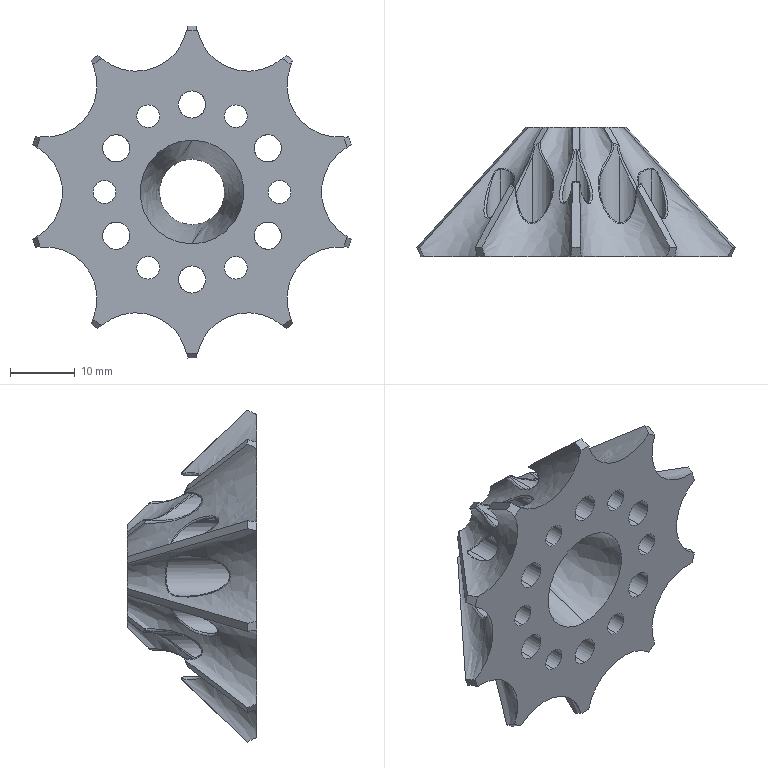Part | SolidWorks | features Chamfer 2, ICE 2, Blend 1, BlendCut 1, Fillet 1 | 1 solid | 122 faces | box 49.123 x 20 x 51.245 mm | volume 9173 mm3 | spline 74 | cylinder 38 | plane 8 | cone 2 | commonest cylinder face diameters 6.3 x14 3.5 x12 4.2 x12